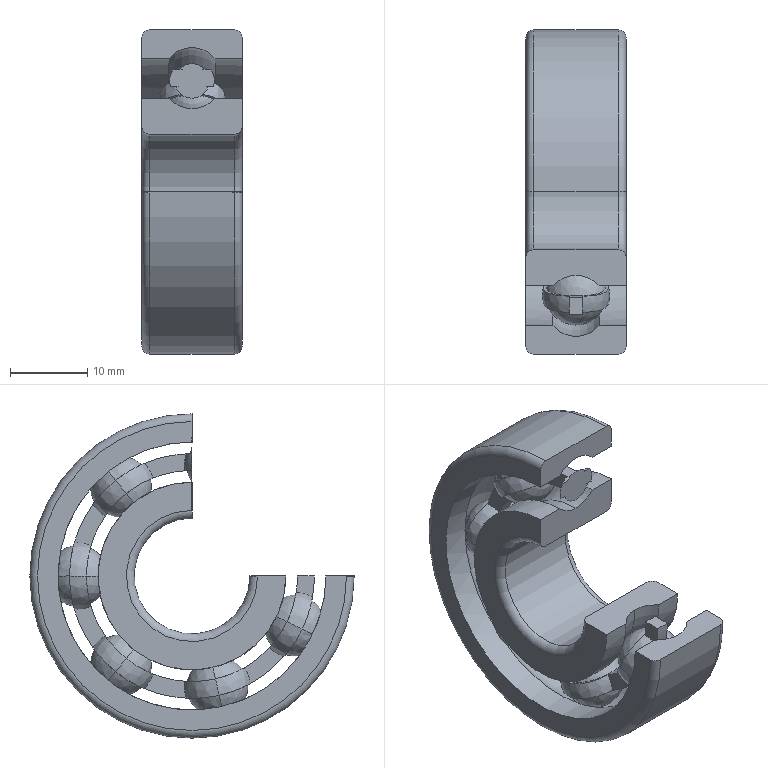Part | STEP file | Bearing 6302 | 1 solid | 96 faces | box 13 x 42 x 42 mm | volume 7777 mm3 | sphere 44 | torus 22 | plane 22 | cylinder 8 | commonest cylinder face diameters 24.3 x2 34.7 x2 15 x1 27.317 x1 31.683 x1 42 x1